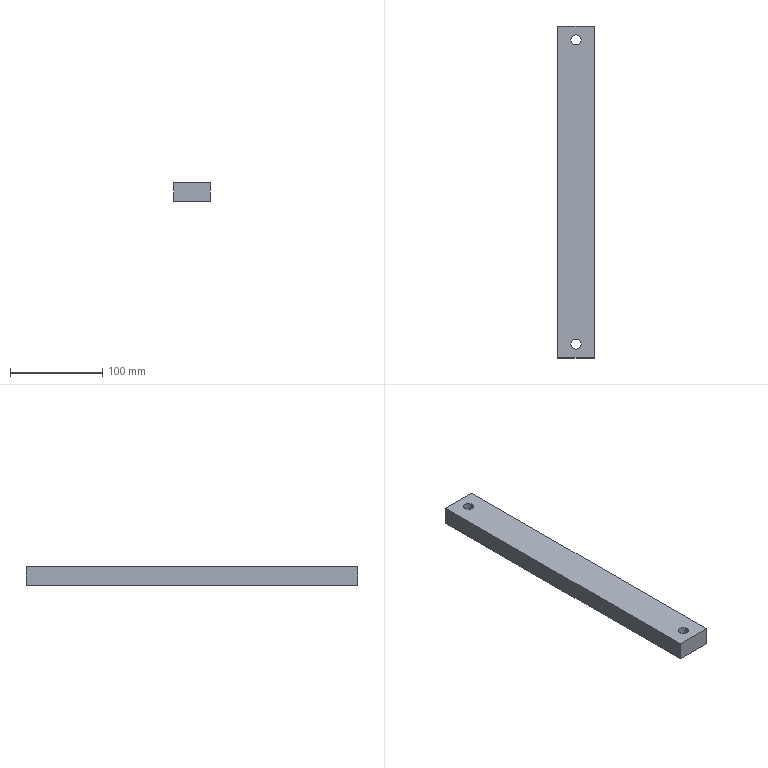Part | STEP file | 1 solid | 12 faces | box 40 x 360 x 20 mm | volume 281296 mm3 | plane 8 | cylinder 4 | commonest cylinder face diameters 11 x2 17 x2
STEP:
#1=CARTESIAN_POINT('',(0.,0.,0.));
#2=DIRECTION('',(0.,0.,1.));
#3=DIRECTION('',(1.,0.,0.));
#4=AXIS2_PLACEMENT_3D('',#1,#2,#3);
#5=CARTESIAN_POINT('',(1352.247,622.48,-145.381));
#6=VERTEX_POINT('',#5);
#7=CARTESIAN_POINT('',(1352.247,262.48,-145.381));
#8=VERTEX_POINT('',#7);
#9=CARTESIAN_POINT('',(1352.247,632.48,-145.381));
#10=DIRECTION('',(0.,-1.,0.));
#11=VECTOR('',#10,1.);
#12=LINE('',#9,#11);
#13=CARTESIAN_POINT('',(1352.247,632.48,-165.381));
#14=DIRECTION('',(-1.,0.,0.));
#15=DIRECTION('',(0.,0.,-1.));
#16=AXIS2_PLACEMENT_3D('',#13,#14,#15);
#17=PLANE('',#16);
#18=CARTESIAN_POINT('',(-20.,0.));
#19=DIRECTION('',(0.,1.));
#20=VECTOR('',#19,1.);
#21=LINE('',#18,#20);
#22=(GEOMETRIC_REPRESENTATION_CONTEXT(2)PARAMETRIC_REPRESENTATION_CONTEXT()REPRESENTATION_CONTEXT('',''));
#23=DEFINITIONAL_REPRESENTATION('',(#21),#22);
#24=PCURVE('',#17,#23);
#25=CARTESIAN_POINT('',(0.,0.,-145.381));
#26=DIRECTION('',(0.,0.,1.));
#27=DIRECTION('',(-1.,0.,0.));
#28=AXIS2_PLACEMENT_3D('',#25,#26,#27);
#29=PLANE('',#28);
#30=CARTESIAN_POINT('',(-1352.247,-632.48));
#31=DIRECTION('',(0.,1.));
#32=VECTOR('',#31,1.);
#33=LINE('',#30,#32);
#34=(GEOMETRIC_REPRESENTATION_CONTEXT(2)PARAMETRIC_REPRESENTATION_CONTEXT()REPRESENTATION_CONTEXT('',''));
#35=DEFINITIONAL_REPRESENTATION('',(#33),#34);
#36=PCURVE('',#29,#35);
#37=SURFACE_CURVE('',#12,(#24,#36),.PCURVE_S1.);
#38=EDGE_CURVE('',#6,#8,#37,.T.);
#39=ORIENTED_EDGE('',*,*,#38,.F.);
#40=CARTESIAN_POINT('',(1352.247,622.48,-165.381));
#41=VERTEX_POINT('',#40);
#42=CARTESIAN_POINT('',(1352.247,622.48,-165.381));
#43=DIRECTION('',(0.,0.,1.));
#44=VECTOR('',#43,1.);
#45=LINE('',#42,#44);
#46=CARTESIAN_POINT('',(0.,10.));
#47=DIRECTION('',(-1.,0.));
#48=VECTOR('',#47,1.);
#49=LINE('',#46,#48);
#50=(GEOMETRIC_REPRESENTATION_CONTEXT(2)PARAMETRIC_REPRESENTATION_CONTEXT()REPRESENTATION_CONTEXT('',''));
#51=DEFINITIONAL_REPRESENTATION('',(#49),#50);
#52=PCURVE('',#17,#51);
#53=CARTESIAN_POINT('',(1392.247,622.48,-165.381));
#54=DIRECTION('',(0.,1.,0.));
#55=DIRECTION('',(0.,0.,-1.));
#56=AXIS2_PLACEMENT_3D('',#53,#54,#55);
#57=PLANE('',#56);
#58=CARTESIAN_POINT('',(0.,40.));
#59=DIRECTION('',(-1.,0.));
#60=VECTOR('',#59,1.);
#61=LINE('',#58,#60);
#62=(GEOMETRIC_REPRESENTATION_CONTEXT(2)PARAMETRIC_REPRESENTATION_CONTEXT()REPRESENTATION_CONTEXT('',''));
#63=DEFINITIONAL_REPRESENTATION('',(#61),#62);
#64=PCURVE('',#57,#63);
#65=SURFACE_CURVE('',#45,(#52,#64),.PCURVE_S1.);
#66=EDGE_CURVE('',#41,#6,#65,.T.);
#67=ORIENTED_EDGE('',*,*,#66,.F.);
#68=CARTESIAN_POINT('',(1352.247,262.48,-165.381));
#69=VERTEX_POINT('',#68);
#70=CARTESIAN_POINT('',(1352.247,0.,-165.381));
#71=DIRECTION('',(0.,-1.,0.));
#72=VECTOR('',#71,1.);
#73=LINE('',#70,#72);
#74=CARTESIAN_POINT('',(0.,632.48));
#75=DIRECTION('',(0.,1.));
#76=VECTOR('',#75,1.);
#77=LINE('',#74,#76);
#78=(GEOMETRIC_REPRESENTATION_CONTEXT(2)PARAMETRIC_REPRESENTATION_CONTEXT()REPRESENTATION_CONTEXT('',''));
#79=DEFINITIONAL_REPRESENTATION('',(#77),#78);
#80=PCURVE('',#17,#79);
#81=CARTESIAN_POINT('',(0.,0.,-165.381));
#82=DIRECTION('',(0.,0.,1.));
#83=DIRECTION('',(-1.,0.,0.));
#84=AXIS2_PLACEMENT_3D('',#81,#82,#83);
#85=PLANE('',#84);
#86=CARTESIAN_POINT('',(-1352.247,0.));
#87=DIRECTION('',(0.,1.));
#88=VECTOR('',#87,1.);
#89=LINE('',#86,#88);
#90=(GEOMETRIC_REPRESENTATION_CONTEXT(2)PARAMETRIC_REPRESENTATION_CONTEXT()REPRESENTATION_CONTEXT('',''));
#91=DEFINITIONAL_REPRESENTATION('',(#89),#90);
#92=PCURVE('',#85,#91);
#93=SURFACE_CURVE('',#73,(#80,#92),.PCURVE_S1.);
#94=EDGE_CURVE('',#41,#69,#93,.T.);
#95=ORIENTED_EDGE('',*,*,#94,.T.);
#96=CARTESIAN_POINT('',(1352.247,262.48,-165.381));
#97=DIRECTION('',(0.,0.,1.));
#98=VECTOR('',#97,1.);
#99=LINE('',#96,#98);
#100=CARTESIAN_POINT('',(0.,370.));
#101=DIRECTION('',(-1.,0.));
#102=VECTOR('',#101,1.);
#103=LINE('',#100,#102);
#104=(GEOMETRIC_REPRESENTATION_CONTEXT(2)PARAMETRIC_REPRESENTATION_CONTEXT()REPRESENTATION_CONTEXT('',''));
#105=DEFINITIONAL_REPRESENTATION('',(#103),#104);
#106=PCURVE('',#17,#105);
#107=CARTESIAN_POINT('',(1352.247,262.48,-165.381));
#108=DIRECTION('',(0.,-1.,0.));
#109=DIRECTION('',(0.,0.,1.));
#110=AXIS2_PLACEMENT_3D('',#107,#108,#109);
#111=PLANE('',#110);
#112=CARTESIAN_POINT('',(0.,0.));
#113=DIRECTION('',(1.,0.));
#114=VECTOR('',#113,1.);
#115=LINE('',#112,#114);
#116=(GEOMETRIC_REPRESENTATION_CONTEXT(2)PARAMETRIC_REPRESENTATION_CONTEXT()REPRESENTATION_CONTEXT('',''));
#117=DEFINITIONAL_REPRESENTATION('',(#115),#116);
#118=PCURVE('',#111,#117);
#119=SURFACE_CURVE('',#99,(#106,#118),.PCURVE_S1.);
#120=EDGE_CURVE('',#69,#8,#119,.T.);
#121=ORIENTED_EDGE('',*,*,#120,.T.);
#122=EDGE_LOOP('',(#39,#67,#95,#121));
#123=FACE_BOUND('',#122,.T.);
#124=ADVANCED_FACE('',(#123),#17,.T.);
#125=CARTESIAN_POINT('',(1392.247,262.48,-145.381));
#126=VERTEX_POINT('',#125);
#127=CARTESIAN_POINT('',(0.,262.48,-145.381));
#128=DIRECTION('',(1.,0.,0.));
#129=VECTOR('',#128,1.);
#130=LINE('',#127,#129);
#131=CARTESIAN_POINT('',(20.,1352.247));
#132=DIRECTION('',(0.,-1.));
#133=VECTOR('',#132,1.);
#134=LINE('',#131,#133);
#135=(GEOMETRIC_REPRESENTATION_CONTEXT(2)PARAMETRIC_REPRESENTATION_CONTEXT()REPRESENTATION_CONTEXT('',''));
#136=DEFINITIONAL_REPRESENTATION('',(#134),#135);
#137=PCURVE('',#111,#136);
#138=CARTESIAN_POINT('',(0.,-262.48));
#139=DIRECTION('',(-1.,0.));
#140=VECTOR('',#139,1.);
#141=LINE('',#138,#140);
#142=(GEOMETRIC_REPRESENTATION_CONTEXT(2)PARAMETRIC_REPRESENTATION_CONTEXT()REPRESENTATION_CONTEXT('',''));
#143=DEFINITIONAL_REPRESENTATION('',(#141),#142);
#144=PCURVE('',#29,#143);
#145=SURFACE_CURVE('',#130,(#137,#144),.PCURVE_S1.);
#146=EDGE_CURVE('',#8,#126,#145,.T.);
#147=ORIENTED_EDGE('',*,*,#146,.F.);
#148=ORIENTED_EDGE('',*,*,#120,.F.);
#149=CARTESIAN_POINT('',(1392.247,262.48,-165.381));
#150=VERTEX_POINT('',#149);
#151=CARTESIAN_POINT('',(0.,262.48,-165.381));
#152=DIRECTION('',(1.,0.,0.));
#153=VECTOR('',#152,1.);
#154=LINE('',#151,#153);
#155=CARTESIAN_POINT('',(0.,1352.247));
#156=DIRECTION('',(0.,-1.));
#157=VECTOR('',#156,1.);
#158=LINE('',#155,#157);
#159=(GEOMETRIC_REPRESENTATION_CONTEXT(2)PARAMETRIC_REPRESENTATION_CONTEXT()REPRESENTATION_CONTEXT('',''));
#160=DEFINITIONAL_REPRESENTATION('',(#158),#159);
#161=PCURVE('',#111,#160);
#162=CARTESIAN_POINT('',(0.,-262.48));
#163=DIRECTION('',(-1.,0.));
#164=VECTOR('',#163,1.);
#165=LINE('',#162,#164);
#166=(GEOMETRIC_REPRESENTATION_CONTEXT(2)PARAMETRIC_REPRESENTATION_CONTEXT()REPRESENTATION_CONTEXT('',''));
#167=DEFINITIONAL_REPRESENTATION('',(#165),#166);
#168=PCURVE('',#85,#167);
#169=SURFACE_CURVE('',#154,(#161,#168),.PCURVE_S1.);
#170=EDGE_CURVE('',#69,#150,#169,.T.);
#171=ORIENTED_EDGE('',*,*,#170,.T.);
#172=CARTESIAN_POINT('',(1392.247,262.48,-165.381));
#173=DIRECTION('',(0.,0.,1.));
#174=VECTOR('',#173,1.);
#175=LINE('',#172,#174);
#176=CARTESIAN_POINT('',(0.,-40.));
#177=DIRECTION('',(1.,0.));
#178=VECTOR('',#177,1.);
#179=LINE('',#176,#178);
#180=(GEOMETRIC_REPRESENTATION_CONTEXT(2)PARAMETRIC_REPRESENTATION_CONTEXT()REPRESENTATION_CONTEXT('',''));
#181=DEFINITIONAL_REPRESENTATION('',(#179),#180);
#182=PCURVE('',#111,#181);
#183=CARTESIAN_POINT('',(1392.247,252.48,-165.381));
#184=DIRECTION('',(1.,0.,0.));
#185=DIRECTION('',(0.,0.,1.));
#186=AXIS2_PLACEMENT_3D('',#183,#184,#185);
#187=PLANE('',#186);
#188=CARTESIAN_POINT('',(0.,-10.));
#189=DIRECTION('',(1.,0.));
#190=VECTOR('',#189,1.);
#191=LINE('',#188,#190);
#192=(GEOMETRIC_REPRESENTATION_CONTEXT(2)PARAMETRIC_REPRESENTATION_CONTEXT()REPRESENTATION_CONTEXT('',''));
#193=DEFINITIONAL_REPRESENTATION('',(#191),#192);
#194=PCURVE('',#187,#193);
#195=SURFACE_CURVE('',#175,(#182,#194),.PCURVE_S1.);
#196=EDGE_CURVE('',#150,#126,#195,.T.);
#197=ORIENTED_EDGE('',*,*,#196,.T.);
#198=EDGE_LOOP('',(#147,#148,#171,#197));
#199=FACE_BOUND('',#198,.T.);
#200=ADVANCED_FACE('',(#199),#111,.T.);
#201=CARTESIAN_POINT('',(1392.247,622.48,-145.381));
#202=VERTEX_POINT('',#201);
#203=CARTESIAN_POINT('',(1392.247,252.48,-145.381));
#204=DIRECTION('',(0.,1.,0.));
#205=VECTOR('',#204,1.);
#206=LINE('',#203,#205);
#207=CARTESIAN_POINT('',(20.,0.));
#208=DIRECTION('',(0.,-1.));
#209=VECTOR('',#208,1.);
#210=LINE('',#207,#209);
#211=(GEOMETRIC_REPRESENTATION_CONTEXT(2)PARAMETRIC_REPRESENTATION_CONTEXT()REPRESENTATION_CONTEXT('',''));
#212=DEFINITIONAL_REPRESENTATION('',(#210),#211);
#213=PCURVE('',#187,#212);
#214=CARTESIAN_POINT('',(-1392.247,-252.48));
#215=DIRECTION('',(0.,-1.));
#216=VECTOR('',#215,1.);
#217=LINE('',#214,#216);
#218=(GEOMETRIC_REPRESENTATION_CONTEXT(2)PARAMETRIC_REPRESENTATION_CONTEXT()REPRESENTATION_CONTEXT('',''));
#219=DEFINITIONAL_REPRESENTATION('',(#217),#218);
#220=PCURVE('',#29,#219);
#221=SURFACE_CURVE('',#206,(#213,#220),.PCURVE_S1.);
#222=EDGE_CURVE('',#126,#202,#221,.T.);
#223=ORIENTED_EDGE('',*,*,#222,.F.);
#224=ORIENTED_EDGE('',*,*,#196,.F.);
#225=CARTESIAN_POINT('',(1392.247,622.48,-165.381));
#226=VERTEX_POINT('',#225);
#227=CARTESIAN_POINT('',(1392.247,0.,-165.381));
#228=DIRECTION('',(0.,1.,0.));
#229=VECTOR('',#228,1.);
#230=LINE('',#227,#229);
#231=CARTESIAN_POINT('',(0.,252.48));
#232=DIRECTION('',(0.,-1.));
#233=VECTOR('',#232,1.);
#234=LINE('',#231,#233);
#235=(GEOMETRIC_REPRESENTATION_CONTEXT(2)PARAMETRIC_REPRESENTATION_CONTEXT()REPRESENTATION_CONTEXT('',''));
#236=DEFINITIONAL_REPRESENTATION('',(#234),#235);
#237=PCURVE('',#187,#236);
#238=CARTESIAN_POINT('',(-1392.247,0.));
#239=DIRECTION('',(0.,-1.));
#240=VECTOR('',#239,1.);
#241=LINE('',#238,#240);
#242=(GEOMETRIC_REPRESENTATION_CONTEXT(2)PARAMETRIC_REPRESENTATION_CONTEXT()REPRESENTATION_CONTEXT('',''));
#243=DEFINITIONAL_REPRESENTATION('',(#241),#242);
#244=PCURVE('',#85,#243);
#245=SURFACE_CURVE('',#230,(#237,#244),.PCURVE_S1.);
#246=EDGE_CURVE('',#150,#226,#245,.T.);
#247=ORIENTED_EDGE('',*,*,#246,.T.);
#248=CARTESIAN_POINT('',(1392.247,622.48,-165.381));
#249=DIRECTION('',(0.,0.,1.));
#250=VECTOR('',#249,1.);
#251=LINE('',#248,#250);
#252=CARTESIAN_POINT('',(0.,-370.));
#253=DIRECTION('',(1.,0.));
#254=VECTOR('',#253,1.);
#255=LINE('',#252,#254);
#256=(GEOMETRIC_REPRESENTATION_CONTEXT(2)PARAMETRIC_REPRESENTATION_CONTEXT()REPRESENTATION_CONTEXT('',''));
#257=DEFINITIONAL_REPRESENTATION('',(#255),#256);
#258=PCURVE('',#187,#257);
#259=CARTESIAN_POINT('',(0.,0.));
#260=DIRECTION('',(-1.,0.));
#261=VECTOR('',#260,1.);
#262=LINE('',#259,#261);
#263=(GEOMETRIC_REPRESENTATION_CONTEXT(2)PARAMETRIC_REPRESENTATION_CONTEXT()REPRESENTATION_CONTEXT('',''));
#264=DEFINITIONAL_REPRESENTATION('',(#262),#263);
#265=PCURVE('',#57,#264);
#266=SURFACE_CURVE('',#251,(#258,#265),.PCURVE_S1.);
#267=EDGE_CURVE('',#226,#202,#266,.T.);
#268=ORIENTED_EDGE('',*,*,#267,.T.);
#269=EDGE_LOOP('',(#223,#224,#247,#268));
#270=FACE_BOUND('',#269,.T.);
#271=ADVANCED_FACE('',(#270),#187,.T.);
#272=CARTESIAN_POINT('',(0.,622.48,-145.381));
#273=DIRECTION('',(-1.,0.,0.));
#274=VECTOR('',#273,1.);
#275=LINE('',#272,#274);
#276=CARTESIAN_POINT('',(-20.,1392.247));
#277=DIRECTION('',(0.,1.));
#278=VECTOR('',#277,1.);
#279=LINE('',#276,#278);
#280=(GEOMETRIC_REPRESENTATION_CONTEXT(2)PARAMETRIC_REPRESENTATION_CONTEXT()REPRESENTATION_CONTEXT('',''));
#281=DEFINITIONAL_REPRESENTATION('',(#279),#280);
#282=PCURVE('',#57,#281);
#283=CARTESIAN_POINT('',(0.,-622.48));
#284=DIRECTION('',(1.,0.));
#285=VECTOR('',#284,1.);
#286=LINE('',#283,#285);
#287=(GEOMETRIC_REPRESENTATION_CONTEXT(2)PARAMETRIC_REPRESENTATION_CONTEXT()REPRESENTATION_CONTEXT('',''));
#288=DEFINITIONAL_REPRESENTATION('',(#286),#287);
#289=PCURVE('',#29,#288);
#290=SURFACE_CURVE('',#275,(#282,#289),.PCURVE_S1.);
#291=EDGE_CURVE('',#202,#6,#290,.T.);
#292=ORIENTED_EDGE('',*,*,#291,.F.);
#293=ORIENTED_EDGE('',*,*,#267,.F.);
#294=CARTESIAN_POINT('',(0.,622.48,-165.381));
#295=DIRECTION('',(-1.,0.,0.));
#296=VECTOR('',#295,1.);
#297=LINE('',#294,#296);
#298=CARTESIAN_POINT('',(0.,1392.247));
#299=DIRECTION('',(0.,1.));
#300=VECTOR('',#299,1.);
#301=LINE('',#298,#300);
#302=(GEOMETRIC_REPRESENTATION_CONTEXT(2)PARAMETRIC_REPRESENTATION_CONTEXT()REPRESENTATION_CONTEXT('',''));
#303=DEFINITIONAL_REPRESENTATION('',(#301),#302);
#304=PCURVE('',#57,#303);
#305=CARTESIAN_POINT('',(0.,-622.48));
#306=DIRECTION('',(1.,0.));
#307=VECTOR('',#306,1.);
#308=LINE('',#305,#307);
#309=(GEOMETRIC_REPRESENTATION_CONTEXT(2)PARAMETRIC_REPRESENTATION_CONTEXT()REPRESENTATION_CONTEXT('',''));
#310=DEFINITIONAL_REPRESENTATION('',(#308),#309);
#311=PCURVE('',#85,#310);
#312=SURFACE_CURVE('',#297,(#304,#311),.PCURVE_S1.);
#313=EDGE_CURVE('',#226,#41,#312,.T.);
#314=ORIENTED_EDGE('',*,*,#313,.T.);
#315=ORIENTED_EDGE('',*,*,#66,.T.);
#316=EDGE_LOOP('',(#292,#293,#314,#315));
#317=FACE_BOUND('',#316,.T.);
#318=ADVANCED_FACE('',(#317),#57,.T.);
#319=CARTESIAN_POINT('',(1380.747,277.48,-165.381));
#320=VERTEX_POINT('',#319);
#321=CARTESIAN_POINT('',(1372.247,277.48,-165.381));
#322=DIRECTION('',(0.,0.,1.));
#323=DIRECTION('',(1.,0.,0.));
#324=AXIS2_PLACEMENT_3D('',#321,#322,#323);
#325=CIRCLE('',#324,8.5);
#326=CARTESIAN_POINT('',(-1372.247,-277.48));
#327=DIRECTION('',(-1.,0.));
#328=AXIS2_PLACEMENT_2D('',#326,#327);
#329=CIRCLE('',#328,8.5);
#330=(GEOMETRIC_REPRESENTATION_CONTEXT(2)PARAMETRIC_REPRESENTATION_CONTEXT()REPRESENTATION_CONTEXT('',''));
#331=DEFINITIONAL_REPRESENTATION('',(#329),#330);
#332=PCURVE('',#85,#331);
#333=CARTESIAN_POINT('',(1372.247,277.48,-170.381));
#334=DIRECTION('',(0.,0.,1.));
#335=DIRECTION('',(-1.,0.,0.));
#336=AXIS2_PLACEMENT_3D('',#333,#334,#335);
#337=CYLINDRICAL_SURFACE('',#336,8.5);
#338=CARTESIAN_POINT('',(3.142,5.));
#339=DIRECTION('',(1.,0.));
#340=VECTOR('',#339,1.);
#341=LINE('',#338,#340);
#342=(GEOMETRIC_REPRESENTATION_CONTEXT(2)PARAMETRIC_REPRESENTATION_CONTEXT()REPRESENTATION_CONTEXT('',''));
#343=DEFINITIONAL_REPRESENTATION('',(#341),#342);
#344=PCURVE('',#337,#343);
#345=SURFACE_CURVE('',#325,(#332,#344),.PCURVE_S1.);
#346=EDGE_CURVE('',#320,#320,#345,.T.);
#347=ORIENTED_EDGE('',*,*,#346,.T.);
#348=EDGE_LOOP('',(#347));
#349=FACE_BOUND('',#348,.T.);
#350=CARTESIAN_POINT('',(1380.747,607.48,-165.381));
#351=VERTEX_POINT('',#350);
#352=CARTESIAN_POINT('',(1372.247,607.48,-165.381));
#353=DIRECTION('',(0.,0.,1.));
#354=DIRECTION('',(1.,0.,0.));
#355=AXIS2_PLACEMENT_3D('',#352,#353,#354);
#356=CIRCLE('',#355,8.5);
#357=CARTESIAN_POINT('',(-1372.247,-607.48));
#358=DIRECTION('',(-1.,0.));
#359=AXIS2_PLACEMENT_2D('',#357,#358);
#360=CIRCLE('',#359,8.5);
#361=(GEOMETRIC_REPRESENTATION_CONTEXT(2)PARAMETRIC_REPRESENTATION_CONTEXT()REPRESENTATION_CONTEXT('',''));
#362=DEFINITIONAL_REPRESENTATION('',(#360),#361);
#363=PCURVE('',#85,#362);
#364=CARTESIAN_POINT('',(1372.247,607.48,-170.381));
#365=DIRECTION('',(0.,0.,1.));
#366=DIRECTION('',(-1.,0.,0.));
#367=AXIS2_PLACEMENT_3D('',#364,#365,#366);
#368=CYLINDRICAL_SURFACE('',#367,8.5);
#369=CARTESIAN_POINT('',(3.142,5.));
#370=DIRECTION('',(1.,0.));
#371=VECTOR('',#370,1.);
#372=LINE('',#369,#371);
#373=(GEOMETRIC_REPRESENTATION_CONTEXT(2)PARAMETRIC_REPRESENTATION_CONTEXT()REPRESENTATION_CONTEXT('',''));
#374=DEFINITIONAL_REPRESENTATION('',(#372),#373);
#375=PCURVE('',#368,#374);
#376=SURFACE_CURVE('',#356,(#363,#375),.PCURVE_S1.);
#377=EDGE_CURVE('',#351,#351,#376,.T.);
#378=ORIENTED_EDGE('',*,*,#377,.T.);
#379=EDGE_LOOP('',(#378));
#380=FACE_BOUND('',#379,.T.);
#381=ORIENTED_EDGE('',*,*,#94,.F.);
#382=ORIENTED_EDGE('',*,*,#313,.F.);
#383=ORIENTED_EDGE('',*,*,#246,.F.);
#384=ORIENTED_EDGE('',*,*,#170,.F.);
#385=EDGE_LOOP('',(#381,#382,#383,#384));
#386=FACE_BOUND('',#385,.T.);
#387=ADVANCED_FACE('',(#349,#380,#386),#85,.F.);
#388=CARTESIAN_POINT('',(1377.747,277.48,-145.381));
#389=VERTEX_POINT('',#388);
#390=CARTESIAN_POINT('',(1372.247,277.48,-145.381));
#391=DIRECTION('',(0.,0.,1.));
#392=DIRECTION('',(1.,0.,0.));
#393=AXIS2_PLACEMENT_3D('',#390,#391,#392);
#394=CIRCLE('',#393,5.5);
#395=CARTESIAN_POINT('',(-1372.247,-277.48));
#396=DIRECTION('',(-1.,0.));
#397=AXIS2_PLACEMENT_2D('',#395,#396);
#398=CIRCLE('',#397,5.5);
#399=(GEOMETRIC_REPRESENTATION_CONTEXT(2)PARAMETRIC_REPRESENTATION_CONTEXT()REPRESENTATION_CONTEXT('',''));
#400=DEFINITIONAL_REPRESENTATION('',(#398),#399);
#401=PCURVE('',#29,#400);
#402=CARTESIAN_POINT('',(1372.247,277.48,-120.381));
#403=DIRECTION('',(0.,0.,1.));
#404=DIRECTION('',(-1.,0.,0.));
#405=AXIS2_PLACEMENT_3D('',#402,#403,#404);
#406=CYLINDRICAL_SURFACE('',#405,5.5);
#407=CARTESIAN_POINT('',(3.142,-25.));
#408=DIRECTION('',(1.,0.));
#409=VECTOR('',#408,1.);
#410=LINE('',#407,#409);
#411=(GEOMETRIC_REPRESENTATION_CONTEXT(2)PARAMETRIC_REPRESENTATION_CONTEXT()REPRESENTATION_CONTEXT('',''));
#412=DEFINITIONAL_REPRESENTATION('',(#410),#411);
#413=PCURVE('',#406,#412);
#414=SURFACE_CURVE('',#394,(#401,#413),.PCURVE_S1.);
#415=EDGE_CURVE('',#389,#389,#414,.T.);
#416=ORIENTED_EDGE('',*,*,#415,.F.);
#417=EDGE_LOOP('',(#416));
#418=FACE_BOUND('',#417,.T.);
#419=CARTESIAN_POINT('',(1377.747,607.48,-145.381));
#420=VERTEX_POINT('',#419);
#421=CARTESIAN_POINT('',(1372.247,607.48,-145.381));
#422=DIRECTION('',(0.,0.,1.));
#423=DIRECTION('',(1.,0.,0.));
#424=AXIS2_PLACEMENT_3D('',#421,#422,#423);
#425=CIRCLE('',#424,5.5);
#426=CARTESIAN_POINT('',(-1372.247,-607.48));
#427=DIRECTION('',(-1.,0.));
#428=AXIS2_PLACEMENT_2D('',#426,#427);
#429=CIRCLE('',#428,5.5);
#430=(GEOMETRIC_REPRESENTATION_CONTEXT(2)PARAMETRIC_REPRESENTATION_CONTEXT()REPRESENTATION_CONTEXT('',''));
#431=DEFINITIONAL_REPRESENTATION('',(#429),#430);
#432=PCURVE('',#29,#431);
#433=CARTESIAN_POINT('',(1372.247,607.48,-120.381));
#434=DIRECTION('',(0.,0.,1.));
#435=DIRECTION('',(-1.,0.,0.));
#436=AXIS2_PLACEMENT_3D('',#433,#434,#435);
#437=CYLINDRICAL_SURFACE('',#436,5.5);
#438=CARTESIAN_POINT('',(3.142,-25.));
#439=DIRECTION('',(1.,0.));
#440=VECTOR('',#439,1.);
#441=LINE('',#438,#440);
#442=(GEOMETRIC_REPRESENTATION_CONTEXT(2)PARAMETRIC_REPRESENTATION_CONTEXT()REPRESENTATION_CONTEXT('',''));
#443=DEFINITIONAL_REPRESENTATION('',(#441),#442);
#444=PCURVE('',#437,#443);
#445=SURFACE_CURVE('',#425,(#432,#444),.PCURVE_S1.);
#446=EDGE_CURVE('',#420,#420,#445,.T.);
#447=ORIENTED_EDGE('',*,*,#446,.F.);
#448=EDGE_LOOP('',(#447));
#449=FACE_BOUND('',#448,.T.);
#450=ORIENTED_EDGE('',*,*,#38,.T.);
#451=ORIENTED_EDGE('',*,*,#146,.T.);
#452=ORIENTED_EDGE('',*,*,#222,.T.);
#453=ORIENTED_EDGE('',*,*,#291,.T.);
#454=EDGE_LOOP('',(#450,#451,#452,#453));
#455=FACE_BOUND('',#454,.T.);
#456=ADVANCED_FACE('',(#418,#449,#455),#29,.T.);
#457=ORIENTED_EDGE('',*,*,#446,.F.);
#458=CARTESIAN_POINT('',(1377.747,607.48,-154.381));
#459=VERTEX_POINT('',#458);
#460=CARTESIAN_POINT('',(1377.747,607.48,-154.381));
#461=CARTESIAN_POINT('',(1377.747,607.48,-145.381));
#462=B_SPLINE_CURVE_WITH_KNOTS('',1,(#460,#461),.UNSPECIFIED.,.F.,.F.,(2,2),(-34.,-25.),.PIECEWISE_BEZIER_KNOTS.);
#463=CARTESIAN_POINT('',(3.142,0.));
#464=DIRECTION('',(0.,1.));
#465=VECTOR('',#464,1.);
#466=LINE('',#463,#465);
#467=(GEOMETRIC_REPRESENTATION_CONTEXT(2)PARAMETRIC_REPRESENTATION_CONTEXT()REPRESENTATION_CONTEXT('',''));
#468=DEFINITIONAL_REPRESENTATION('',(#466),#467);
#469=PCURVE('',#437,#468);
#470=CARTESIAN_POINT('',(9.425,0.));
#471=DIRECTION('',(0.,1.));
#472=VECTOR('',#471,1.);
#473=LINE('',#470,#472);
#474=(GEOMETRIC_REPRESENTATION_CONTEXT(2)PARAMETRIC_REPRESENTATION_CONTEXT()REPRESENTATION_CONTEXT('',''));
#475=DEFINITIONAL_REPRESENTATION('',(#473),#474);
#476=PCURVE('',#437,#475);
#477=SEAM_CURVE('',#462,(#469,#476),.PCURVE_S1.);
#478=EDGE_CURVE('',#459,#420,#477,.T.);
#479=ORIENTED_EDGE('',*,*,#478,.F.);
#480=CARTESIAN_POINT('',(1372.247,607.48,-154.381));
#481=DIRECTION('',(0.,0.,-1.));
#482=DIRECTION('',(1.,0.,0.));
#483=AXIS2_PLACEMENT_3D('',#480,#481,#482);
#484=CIRCLE('',#483,5.5);
#485=CARTESIAN_POINT('',(9.425,-34.));
#486=DIRECTION('',(-1.,0.));
#487=VECTOR('',#486,1.);
#488=LINE('',#485,#487);
#489=(GEOMETRIC_REPRESENTATION_CONTEXT(2)PARAMETRIC_REPRESENTATION_CONTEXT()REPRESENTATION_CONTEXT('',''));
#490=DEFINITIONAL_REPRESENTATION('',(#488),#489);
#491=PCURVE('',#437,#490);
#492=CARTESIAN_POINT('',(1372.247,607.48,-154.381));
#493=DIRECTION('',(0.,0.,1.));
#494=DIRECTION('',(-1.,0.,0.));
#495=AXIS2_PLACEMENT_3D('',#492,#493,#494);
#496=PLANE('',#495);
#497=CARTESIAN_POINT('',(-5.5,0.));
#498=CARTESIAN_POINT('',(-5.5,9.526));
#499=CARTESIAN_POINT('',(2.75,4.763));
#500=CARTESIAN_POINT('',(11.,0.));
#501=CARTESIAN_POINT('',(2.75,-4.763));
#502=CARTESIAN_POINT('',(-5.5,-9.526));
#503=CARTESIAN_POINT('',(-5.5,0.));
#504=(BOUNDED_CURVE()B_SPLINE_CURVE(2,(#497,#498,#499,#500,#501,#502,#503),.UNSPECIFIED.,.T.,.F.)B_SPLINE_CURVE_WITH_KNOTS((1,2,2,2,2,1),(-2.094,0.,2.094,4.189,6.283,8.378),.UNSPECIFIED.)CURVE()GEOMETRIC_REPRESENTATION_ITEM()RATIONAL_B_SPLINE_CURVE((1.,0.5,1.,0.5,1.,0.5,1.))REPRESENTATION_ITEM(''));
#505=(GEOMETRIC_REPRESENTATION_CONTEXT(2)PARAMETRIC_REPRESENTATION_CONTEXT()REPRESENTATION_CONTEXT('',''));
#506=DEFINITIONAL_REPRESENTATION('',(#504),#505);
#507=PCURVE('',#496,#506);
#508=SURFACE_CURVE('',#484,(#491,#507),.PCURVE_S1.);
#509=EDGE_CURVE('',#459,#459,#508,.T.);
#510=ORIENTED_EDGE('',*,*,#509,.F.);
#511=ORIENTED_EDGE('',*,*,#478,.T.);
#512=EDGE_LOOP('',(#457,#479,#510,#511));
#513=FACE_BOUND('',#512,.F.);
#514=ADVANCED_FACE('',(#513),#437,.F.);
#515=ORIENTED_EDGE('',*,*,#509,.F.);
#516=EDGE_LOOP('',(#515));
#517=FACE_BOUND('',#516,.T.);
#518=CARTESIAN_POINT('',(1380.747,607.48,-154.381));
#519=VERTEX_POINT('',#518);
#520=CARTESIAN_POINT('',(1372.247,607.48,-154.381));
#521=DIRECTION('',(0.,0.,-1.));
#522=DIRECTION('',(1.,0.,0.));
#523=AXIS2_PLACEMENT_3D('',#520,#521,#522);
#524=CIRCLE('',#523,8.5);
#525=CARTESIAN_POINT('',(-8.5,0.));
#526=CARTESIAN_POINT('',(-8.5,14.722));
#527=CARTESIAN_POINT('',(4.25,7.361));
#528=CARTESIAN_POINT('',(17.,0.));
#529=CARTESIAN_POINT('',(4.25,-7.361));
#530=CARTESIAN_POINT('',(-8.5,-14.722));
#531=CARTESIAN_POINT('',(-8.5,0.));
#532=(BOUNDED_CURVE()B_SPLINE_CURVE(2,(#525,#526,#527,#528,#529,#530,#531),.UNSPECIFIED.,.T.,.F.)B_SPLINE_CURVE_WITH_KNOTS((1,2,2,2,2,1),(-2.094,0.,2.094,4.189,6.283,8.378),.UNSPECIFIED.)CURVE()GEOMETRIC_REPRESENTATION_ITEM()RATIONAL_B_SPLINE_CURVE((1.,0.5,1.,0.5,1.,0.5,1.))REPRESENTATION_ITEM(''));
#533=(GEOMETRIC_REPRESENTATION_CONTEXT(2)PARAMETRIC_REPRESENTATION_CONTEXT()REPRESENTATION_CONTEXT('',''));
#534=DEFINITIONAL_REPRESENTATION('',(#532),#533);
#535=PCURVE('',#496,#534);
#536=CARTESIAN_POINT('',(9.425,16.));
#537=DIRECTION('',(-1.,0.));
#538=VECTOR('',#537,1.);
#539=LINE('',#536,#538);
#540=(GEOMETRIC_REPRESENTATION_CONTEXT(2)PARAMETRIC_REPRESENTATION_CONTEXT()REPRESENTATION_CONTEXT('',''));
#541=DEFINITIONAL_REPRESENTATION('',(#539),#540);
#542=PCURVE('',#368,#541);
#543=SURFACE_CURVE('',#524,(#535,#542),.PCURVE_S1.);
#544=EDGE_CURVE('',#519,#519,#543,.T.);
#545=ORIENTED_EDGE('',*,*,#544,.T.);
#546=EDGE_LOOP('',(#545));
#547=FACE_BOUND('',#546,.T.);
#548=ADVANCED_FACE('',(#517,#547),#496,.F.);
#549=ORIENTED_EDGE('',*,*,#544,.T.);
#550=CARTESIAN_POINT('',(1380.747,607.48,-165.381));
#551=CARTESIAN_POINT('',(1380.747,607.48,-154.381));
#552=B_SPLINE_CURVE_WITH_KNOTS('',1,(#550,#551),.UNSPECIFIED.,.F.,.F.,(2,2),(5.,16.),.PIECEWISE_BEZIER_KNOTS.);
#553=CARTESIAN_POINT('',(3.142,0.));
#554=DIRECTION('',(0.,1.));
#555=VECTOR('',#554,1.);
#556=LINE('',#553,#555);
#557=(GEOMETRIC_REPRESENTATION_CONTEXT(2)PARAMETRIC_REPRESENTATION_CONTEXT()REPRESENTATION_CONTEXT('',''));
#558=DEFINITIONAL_REPRESENTATION('',(#556),#557);
#559=PCURVE('',#368,#558);
#560=CARTESIAN_POINT('',(9.425,0.));
#561=DIRECTION('',(0.,1.));
#562=VECTOR('',#561,1.);
#563=LINE('',#560,#562);
#564=(GEOMETRIC_REPRESENTATION_CONTEXT(2)PARAMETRIC_REPRESENTATION_CONTEXT()REPRESENTATION_CONTEXT('',''));
#565=DEFINITIONAL_REPRESENTATION('',(#563),#564);
#566=PCURVE('',#368,#565);
#567=SEAM_CURVE('',#552,(#559,#566),.PCURVE_S1.);
#568=EDGE_CURVE('',#351,#519,#567,.T.);
#569=ORIENTED_EDGE('',*,*,#568,.F.);
#570=ORIENTED_EDGE('',*,*,#377,.T.);
#571=ORIENTED_EDGE('',*,*,#568,.T.);
#572=EDGE_LOOP('',(#549,#569,#570,#571));
#573=FACE_BOUND('',#572,.F.);
#574=ADVANCED_FACE('',(#573),#368,.F.);
#575=ORIENTED_EDGE('',*,*,#415,.F.);
#576=CARTESIAN_POINT('',(1377.747,277.48,-154.381));
#577=VERTEX_POINT('',#576);
#578=CARTESIAN_POINT('',(1377.747,277.48,-154.381));
#579=CARTESIAN_POINT('',(1377.747,277.48,-145.381));
#580=B_SPLINE_CURVE_WITH_KNOTS('',1,(#578,#579),.UNSPECIFIED.,.F.,.F.,(2,2),(-34.,-25.),.PIECEWISE_BEZIER_KNOTS.);
#581=CARTESIAN_POINT('',(3.142,0.));
#582=DIRECTION('',(0.,1.));
#583=VECTOR('',#582,1.);
#584=LINE('',#581,#583);
#585=(GEOMETRIC_REPRESENTATION_CONTEXT(2)PARAMETRIC_REPRESENTATION_CONTEXT()REPRESENTATION_CONTEXT('',''));
#586=DEFINITIONAL_REPRESENTATION('',(#584),#585);
#587=PCURVE('',#406,#586);
#588=CARTESIAN_POINT('',(9.425,0.));
#589=DIRECTION('',(0.,1.));
#590=VECTOR('',#589,1.);
#591=LINE('',#588,#590);
#592=(GEOMETRIC_REPRESENTATION_CONTEXT(2)PARAMETRIC_REPRESENTATION_CONTEXT()REPRESENTATION_CONTEXT('',''));
#593=DEFINITIONAL_REPRESENTATION('',(#591),#592);
#594=PCURVE('',#406,#593);
#595=SEAM_CURVE('',#580,(#587,#594),.PCURVE_S1.);
#596=EDGE_CURVE('',#577,#389,#595,.T.);
#597=ORIENTED_EDGE('',*,*,#596,.F.);
#598=CARTESIAN_POINT('',(1372.247,277.48,-154.381));
#599=DIRECTION('',(0.,0.,-1.));
#600=DIRECTION('',(1.,0.,0.));
#601=AXIS2_PLACEMENT_3D('',#598,#599,#600);
#602=CIRCLE('',#601,5.5);
#603=CARTESIAN_POINT('',(9.425,-34.));
#604=DIRECTION('',(-1.,0.));
#605=VECTOR('',#604,1.);
#606=LINE('',#603,#605);
#607=(GEOMETRIC_REPRESENTATION_CONTEXT(2)PARAMETRIC_REPRESENTATION_CONTEXT()REPRESENTATION_CONTEXT('',''));
#608=DEFINITIONAL_REPRESENTATION('',(#606),#607);
#609=PCURVE('',#406,#608);
#610=CARTESIAN_POINT('',(1372.247,277.48,-154.381));
#611=DIRECTION('',(0.,0.,1.));
#612=DIRECTION('',(-1.,0.,0.));
#613=AXIS2_PLACEMENT_3D('',#610,#611,#612);
#614=PLANE('',#613);
#615=CARTESIAN_POINT('',(-5.5,0.));
#616=CARTESIAN_POINT('',(-5.5,9.526));
#617=CARTESIAN_POINT('',(2.75,4.763));
#618=CARTESIAN_POINT('',(11.,0.));
#619=CARTESIAN_POINT('',(2.75,-4.763));
#620=CARTESIAN_POINT('',(-5.5,-9.526));
#621=CARTESIAN_POINT('',(-5.5,0.));
#622=(BOUNDED_CURVE()B_SPLINE_CURVE(2,(#615,#616,#617,#618,#619,#620,#621),.UNSPECIFIED.,.T.,.F.)B_SPLINE_CURVE_WITH_KNOTS((1,2,2,2,2,1),(-2.094,0.,2.094,4.189,6.283,8.378),.UNSPECIFIED.)CURVE()GEOMETRIC_REPRESENTATION_ITEM()RATIONAL_B_SPLINE_CURVE((1.,0.5,1.,0.5,1.,0.5,1.))REPRESENTATION_ITEM(''));
#623=(GEOMETRIC_REPRESENTATION_CONTEXT(2)PARAMETRIC_REPRESENTATION_CONTEXT()REPRESENTATION_CONTEXT('',''));
#624=DEFINITIONAL_REPRESENTATION('',(#622),#623);
#625=PCURVE('',#614,#624);
#626=SURFACE_CURVE('',#602,(#609,#625),.PCURVE_S1.);
#627=EDGE_CURVE('',#577,#577,#626,.T.);
#628=ORIENTED_EDGE('',*,*,#627,.F.);
#629=ORIENTED_EDGE('',*,*,#596,.T.);
#630=EDGE_LOOP('',(#575,#597,#628,#629));
#631=FACE_BOUND('',#630,.F.);
#632=ADVANCED_FACE('',(#631),#406,.F.);
#633=ORIENTED_EDGE('',*,*,#627,.F.);
#634=EDGE_LOOP('',(#633));
#635=FACE_BOUND('',#634,.T.);
#636=CARTESIAN_POINT('',(1380.747,277.48,-154.381));
#637=VERTEX_POINT('',#636);
#638=CARTESIAN_POINT('',(1372.247,277.48,-154.381));
#639=DIRECTION('',(0.,0.,-1.));
#640=DIRECTION('',(1.,0.,0.));
#641=AXIS2_PLACEMENT_3D('',#638,#639,#640);
#642=CIRCLE('',#641,8.5);
#643=CARTESIAN_POINT('',(-8.5,0.));
#644=CARTESIAN_POINT('',(-8.5,14.722));
#645=CARTESIAN_POINT('',(4.25,7.361));
#646=CARTESIAN_POINT('',(17.,0.));
#647=CARTESIAN_POINT('',(4.25,-7.361));
#648=CARTESIAN_POINT('',(-8.5,-14.722));
#649=CARTESIAN_POINT('',(-8.5,0.));
#650=(BOUNDED_CURVE()B_SPLINE_CURVE(2,(#643,#644,#645,#646,#647,#648,#649),.UNSPECIFIED.,.T.,.F.)B_SPLINE_CURVE_WITH_KNOTS((1,2,2,2,2,1),(-2.094,0.,2.094,4.189,6.283,8.378),.UNSPECIFIED.)CURVE()GEOMETRIC_REPRESENTATION_ITEM()RATIONAL_B_SPLINE_CURVE((1.,0.5,1.,0.5,1.,0.5,1.))REPRESENTATION_ITEM(''));
#651=(GEOMETRIC_REPRESENTATION_CONTEXT(2)PARAMETRIC_REPRESENTATION_CONTEXT()REPRESENTATION_CONTEXT('',''));
#652=DEFINITIONAL_REPRESENTATION('',(#650),#651);
#653=PCURVE('',#614,#652);
#654=CARTESIAN_POINT('',(9.425,16.));
#655=DIRECTION('',(-1.,0.));
#656=VECTOR('',#655,1.);
#657=LINE('',#654,#656);
#658=(GEOMETRIC_REPRESENTATION_CONTEXT(2)PARAMETRIC_REPRESENTATION_CONTEXT()REPRESENTATION_CONTEXT('',''));
#659=DEFINITIONAL_REPRESENTATION('',(#657),#658);
#660=PCURVE('',#337,#659);
#661=SURFACE_CURVE('',#642,(#653,#660),.PCURVE_S1.);
#662=EDGE_CURVE('',#637,#637,#661,.T.);
#663=ORIENTED_EDGE('',*,*,#662,.T.);
#664=EDGE_LOOP('',(#663));
#665=FACE_BOUND('',#664,.T.);
#666=ADVANCED_FACE('',(#635,#665),#614,.F.);
#667=ORIENTED_EDGE('',*,*,#662,.T.);
#668=CARTESIAN_POINT('',(1380.747,277.48,-165.381));
#669=CARTESIAN_POINT('',(1380.747,277.48,-154.381));
#670=B_SPLINE_CURVE_WITH_KNOTS('',1,(#668,#669),.UNSPECIFIED.,.F.,.F.,(2,2),(5.,16.),.PIECEWISE_BEZIER_KNOTS.);
#671=CARTESIAN_POINT('',(3.142,0.));
#672=DIRECTION('',(0.,1.));
#673=VECTOR('',#672,1.);
#674=LINE('',#671,#673);
#675=(GEOMETRIC_REPRESENTATION_CONTEXT(2)PARAMETRIC_REPRESENTATION_CONTEXT()REPRESENTATION_CONTEXT('',''));
#676=DEFINITIONAL_REPRESENTATION('',(#674),#675);
#677=PCURVE('',#337,#676);
#678=CARTESIAN_POINT('',(9.425,0.));
#679=DIRECTION('',(0.,1.));
#680=VECTOR('',#679,1.);
#681=LINE('',#678,#680);
#682=(GEOMETRIC_REPRESENTATION_CONTEXT(2)PARAMETRIC_REPRESENTATION_CONTEXT()REPRESENTATION_CONTEXT('',''));
#683=DEFINITIONAL_REPRESENTATION('',(#681),#682);
#684=PCURVE('',#337,#683);
#685=SEAM_CURVE('',#670,(#677,#684),.PCURVE_S1.);
#686=EDGE_CURVE('',#320,#637,#685,.T.);
#687=ORIENTED_EDGE('',*,*,#686,.F.);
#688=ORIENTED_EDGE('',*,*,#346,.T.);
#689=ORIENTED_EDGE('',*,*,#686,.T.);
#690=EDGE_LOOP('',(#667,#687,#688,#689));
#691=FACE_BOUND('',#690,.F.);
#692=ADVANCED_FACE('',(#691),#337,.F.);
#693=CLOSED_SHELL('',(#124,#200,#271,#318,#387,#456,#514,#548,#574,#632,#666,#692));
#694=MANIFOLD_SOLID_BREP('',#693);
#695=(LENGTH_UNIT()NAMED_UNIT(*)SI_UNIT(.MILLI.,.METRE.));
#696=UNCERTAINTY_MEASURE_WITH_UNIT(LENGTH_MEASURE(0.000005),#695,'','');
#697=(NAMED_UNIT(*)PLANE_ANGLE_UNIT()SI_UNIT($,.RADIAN.));
#698=(NAMED_UNIT(*)SI_UNIT($,.STERADIAN.)SOLID_ANGLE_UNIT());
#699=(GEOMETRIC_REPRESENTATION_CONTEXT(3)GLOBAL_UNCERTAINTY_ASSIGNED_CONTEXT((#696))GLOBAL_UNIT_ASSIGNED_CONTEXT((#695,#697,#698))REPRESENTATION_CONTEXT('',''));
#700=ADVANCED_BREP_SHAPE_REPRESENTATION('',(#4,#694),#699);